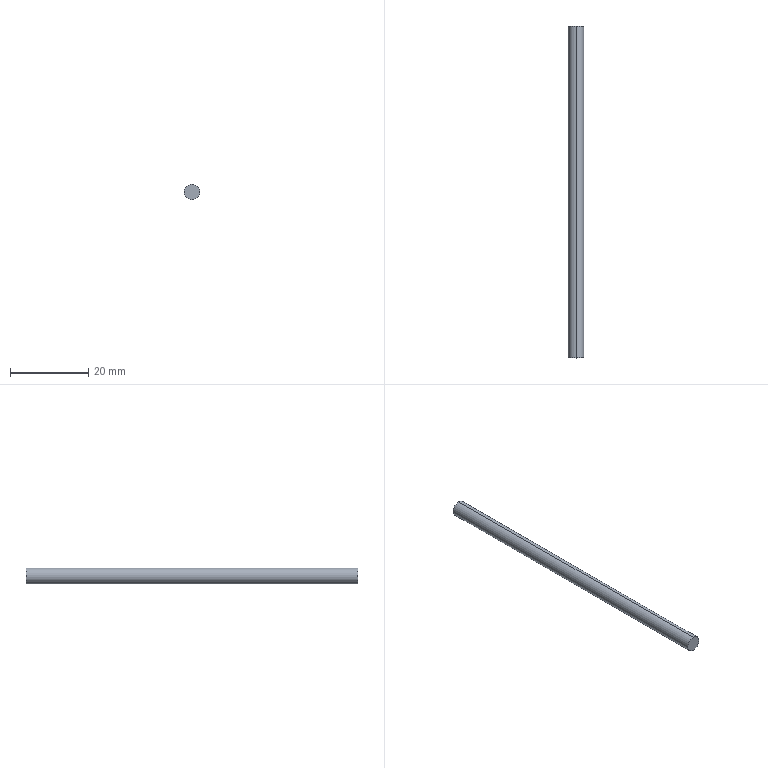Part | SolidWorks | features Extrusion 1 | 1 solid | 4 faces | box 4 x 85 x 4 mm | volume 1068 mm3 | cylinder 2 | plane 2 | commonest cylinder face diameters 4 x2
STEP:
#1=CARTESIAN_POINT('',(0.,85.,2.));
#2=VERTEX_POINT('',#1);
#3=CARTESIAN_POINT('',(0.,85.,-2.));
#4=VERTEX_POINT('',#3);
#5=CARTESIAN_POINT('',(0.,85.,0.));
#6=DIRECTION('',(0.,1.,0.));
#7=DIRECTION('',(0.,0.,1.));
#8=AXIS2_PLACEMENT_3D('',#5,#6,#7);
#9=CIRCLE('',#8,2.);
#10=EDGE_CURVE('',#2,#4,#9,.T.);
#11=ORIENTED_EDGE('',*,*,#10,.F.);
#12=CARTESIAN_POINT('',(0.,0.,2.));
#13=VERTEX_POINT('',#12);
#14=CARTESIAN_POINT('',(0.,85.,2.));
#15=DIRECTION('',(0.,-1.,0.));
#16=VECTOR('',#15,1000.);
#17=LINE('',#14,#16);
#18=EDGE_CURVE('',#2,#13,#17,.T.);
#19=ORIENTED_EDGE('',*,*,#18,.T.);
#20=CARTESIAN_POINT('',(0.,0.,-2.));
#21=VERTEX_POINT('',#20);
#22=CARTESIAN_POINT('',(0.,0.,0.));
#23=DIRECTION('',(0.,1.,0.));
#24=DIRECTION('',(0.,0.,1.));
#25=AXIS2_PLACEMENT_3D('',#22,#23,#24);
#26=CIRCLE('',#25,2.);
#27=EDGE_CURVE('',#13,#21,#26,.T.);
#28=ORIENTED_EDGE('',*,*,#27,.T.);
#29=CARTESIAN_POINT('',(0.,85.,-2.));
#30=DIRECTION('',(0.,-1.,0.));
#31=VECTOR('',#30,1000.);
#32=LINE('',#29,#31);
#33=EDGE_CURVE('',#4,#21,#32,.T.);
#34=ORIENTED_EDGE('',*,*,#33,.F.);
#35=EDGE_LOOP('',(#11,#19,#28,#34));
#36=FACE_OUTER_BOUND('',#35,.T.);
#37=CARTESIAN_POINT('',(0.,85.,0.));
#38=DIRECTION('',(0.,-1.,0.));
#39=DIRECTION('',(0.,0.,-1.));
#40=AXIS2_PLACEMENT_3D('',#37,#38,#39);
#41=CYLINDRICAL_SURFACE('',#40,2.);
#42=ADVANCED_FACE('',(#36),#41,.T.);
#43=ORIENTED_EDGE('',*,*,#18,.F.);
#44=CARTESIAN_POINT('',(0.,85.,0.));
#45=DIRECTION('',(0.,1.,0.));
#46=DIRECTION('',(0.,0.,1.));
#47=AXIS2_PLACEMENT_3D('',#44,#45,#46);
#48=CIRCLE('',#47,2.);
#49=EDGE_CURVE('',#4,#2,#48,.T.);
#50=ORIENTED_EDGE('',*,*,#49,.F.);
#51=ORIENTED_EDGE('',*,*,#33,.T.);
#52=CARTESIAN_POINT('',(0.,0.,0.));
#53=DIRECTION('',(0.,1.,0.));
#54=DIRECTION('',(0.,0.,1.));
#55=AXIS2_PLACEMENT_3D('',#52,#53,#54);
#56=CIRCLE('',#55,2.);
#57=EDGE_CURVE('',#21,#13,#56,.T.);
#58=ORIENTED_EDGE('',*,*,#57,.T.);
#59=EDGE_LOOP('',(#43,#50,#51,#58));
#60=FACE_OUTER_BOUND('',#59,.T.);
#61=CARTESIAN_POINT('',(0.,85.,0.));
#62=DIRECTION('',(0.,-1.,0.));
#63=DIRECTION('',(0.,0.,-1.));
#64=AXIS2_PLACEMENT_3D('',#61,#62,#63);
#65=CYLINDRICAL_SURFACE('',#64,2.);
#66=ADVANCED_FACE('',(#60),#65,.T.);
#67=ORIENTED_EDGE('',*,*,#49,.T.);
#68=ORIENTED_EDGE('',*,*,#10,.T.);
#69=EDGE_LOOP('',(#67,#68));
#70=FACE_OUTER_BOUND('',#69,.T.);
#71=CARTESIAN_POINT('',(0.,85.,0.));
#72=DIRECTION('',(0.,1.,0.));
#73=DIRECTION('',(0.,0.,1.));
#74=AXIS2_PLACEMENT_3D('',#71,#72,#73);
#75=PLANE('',#74);
#76=ADVANCED_FACE('',(#70),#75,.T.);
#77=ORIENTED_EDGE('',*,*,#57,.F.);
#78=ORIENTED_EDGE('',*,*,#27,.F.);
#79=EDGE_LOOP('',(#77,#78));
#80=FACE_OUTER_BOUND('',#79,.T.);
#81=CARTESIAN_POINT('',(0.,0.,0.));
#82=DIRECTION('',(0.,1.,0.));
#83=DIRECTION('',(0.,0.,1.));
#84=AXIS2_PLACEMENT_3D('',#81,#82,#83);
#85=PLANE('',#84);
#86=ADVANCED_FACE('',(#80),#85,.F.);
#87=CLOSED_SHELL('',(#42,#66,#76,#86));
#88=MANIFOLD_SOLID_BREP('',#87);
#89=CARTESIAN_POINT('',(0.,0.,0.));
#90=DIRECTION('',(0.,0.,1.));
#91=DIRECTION('',(1.,0.,0.));
#92=AXIS2_PLACEMENT_3D('',#89,#90,#91);
#93=(LENGTH_UNIT()NAMED_UNIT(*)SI_UNIT(.MILLI.,.METRE.));
#94=UNCERTAINTY_MEASURE_WITH_UNIT(LENGTH_MEASURE(0.00001),#93,'','');
#95=(NAMED_UNIT(*)PLANE_ANGLE_UNIT()SI_UNIT($,.RADIAN.));
#96=(NAMED_UNIT(*)SI_UNIT($,.STERADIAN.)SOLID_ANGLE_UNIT());
#97=(GEOMETRIC_REPRESENTATION_CONTEXT(3)GLOBAL_UNCERTAINTY_ASSIGNED_CONTEXT((#94))GLOBAL_UNIT_ASSIGNED_CONTEXT((#93,#95,#96))REPRESENTATION_CONTEXT('',''));
#98=ADVANCED_BREP_SHAPE_REPRESENTATION('',(#88,#92),#97);